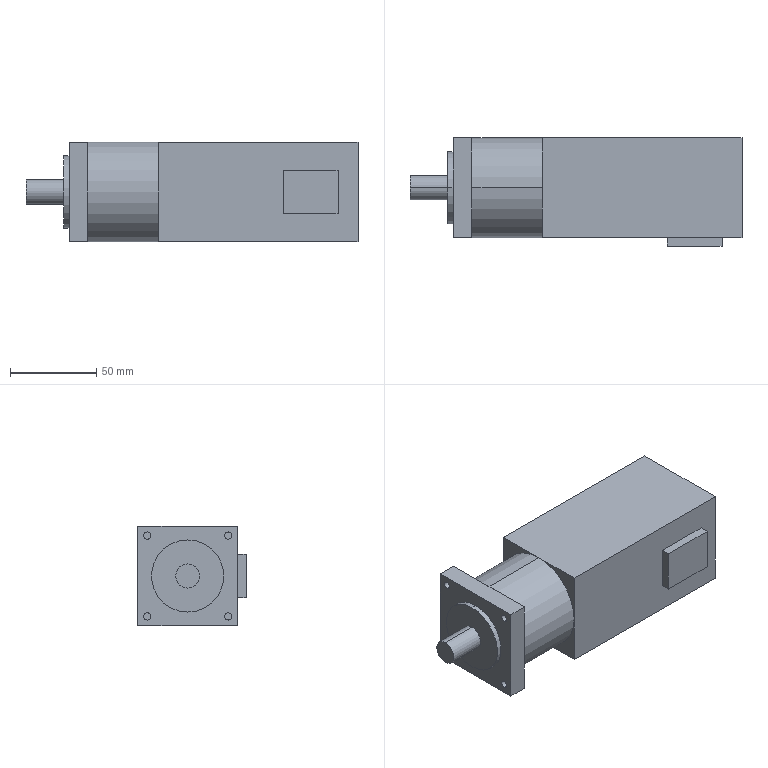Part | STEP file | PX57N005S0 planetary reducer+motor V1.201001 | 1 solid | 39 faces | box 193 x 63 x 58 mm | volume 546492 mm3 | plane 25 | cylinder 14 | commonest cylinder face diameters 4.2 x8 14 x2 42 x2 58 x2